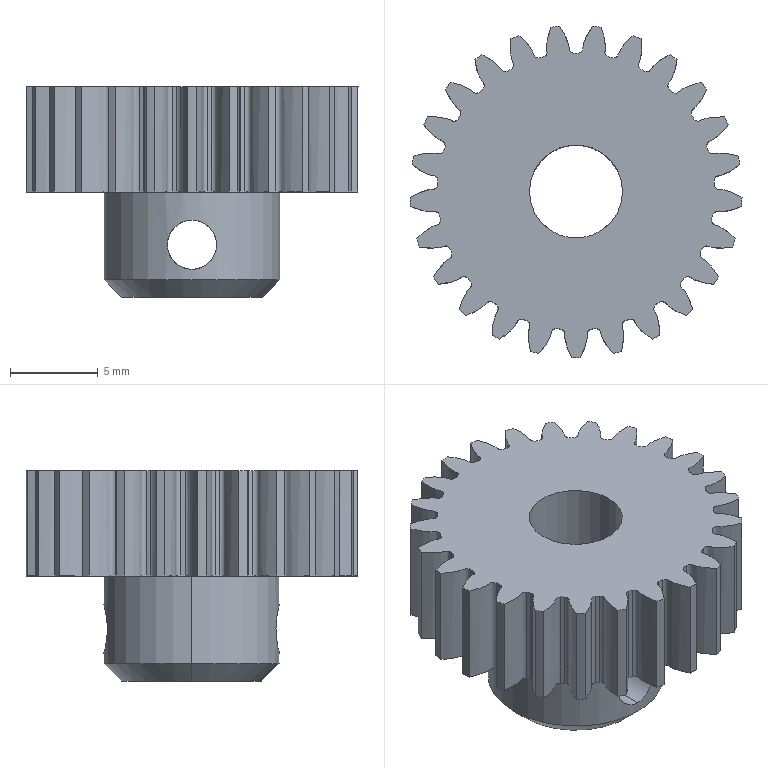Part | SolidWorks | features ICE 6, Chamfer 1, CirPattern 1, Extrusion 1, RefAxis 1 | 1 solid | 113 faces | box 18.888 x 18.854 x 12 mm | volume 1581 mm3 | cylinder 58 | spline 50 | plane 3 | cone 2 | commonest cylinder face diameters 15.75 x25 18.9 x25 2.8 x4 5.3 x2 10 x2